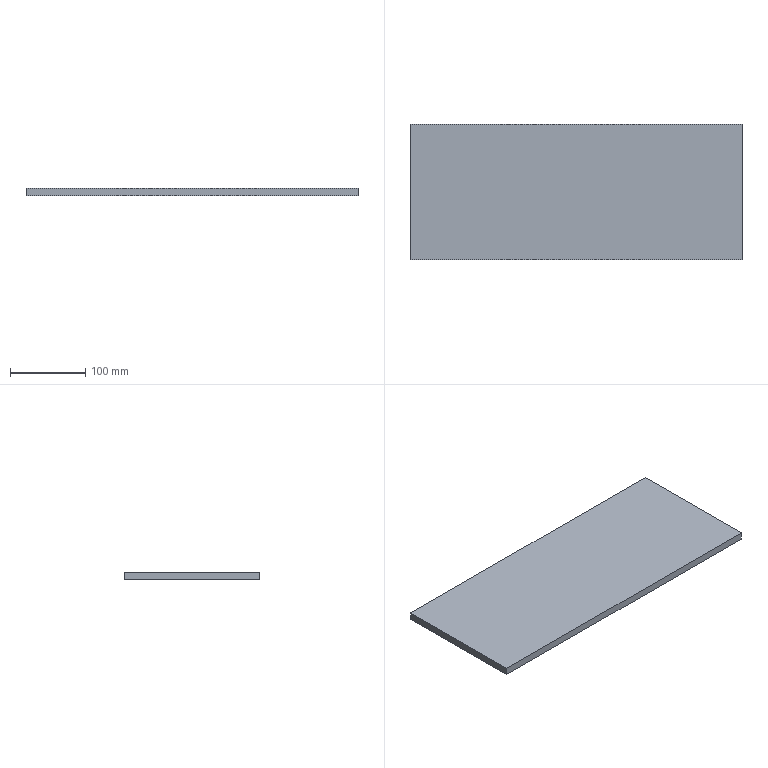Part | SolidWorks | features Extrusion 1 | 1 solid | 6 faces | box 440 x 180 x 10 mm | volume 792000 mm3 | plane 6
STEP:
#1=CARTESIAN_POINT('',(0.,0.,0.));
#2=VERTEX_POINT('',#1);
#3=CARTESIAN_POINT('',(0.,-180.,0.));
#4=VERTEX_POINT('',#3);
#5=CARTESIAN_POINT('',(0.,-180.,0.));
#6=DIRECTION('',(0.,-1.,0.));
#7=VECTOR('',#6,1000.);
#8=LINE('',#5,#7);
#9=EDGE_CURVE('',#2,#4,#8,.T.);
#10=ORIENTED_EDGE('',*,*,#9,.T.);
#11=CARTESIAN_POINT('',(0.,-180.,10.));
#12=VERTEX_POINT('',#11);
#13=CARTESIAN_POINT('',(0.,-180.,10.));
#14=DIRECTION('',(0.,0.,-1.));
#15=VECTOR('',#14,1000.);
#16=LINE('',#13,#15);
#17=EDGE_CURVE('',#12,#4,#16,.T.);
#18=ORIENTED_EDGE('',*,*,#17,.F.);
#19=CARTESIAN_POINT('',(0.,0.,10.));
#20=VERTEX_POINT('',#19);
#21=CARTESIAN_POINT('',(0.,-180.,10.));
#22=DIRECTION('',(0.,-1.,0.));
#23=VECTOR('',#22,1000.);
#24=LINE('',#21,#23);
#25=EDGE_CURVE('',#20,#12,#24,.T.);
#26=ORIENTED_EDGE('',*,*,#25,.F.);
#27=CARTESIAN_POINT('',(0.,0.,10.));
#28=DIRECTION('',(0.,0.,-1.));
#29=VECTOR('',#28,1000.);
#30=LINE('',#27,#29);
#31=EDGE_CURVE('',#20,#2,#30,.T.);
#32=ORIENTED_EDGE('',*,*,#31,.T.);
#33=EDGE_LOOP('',(#10,#18,#26,#32));
#34=FACE_OUTER_BOUND('',#33,.T.);
#35=CARTESIAN_POINT('',(0.,-180.,10.));
#36=DIRECTION('',(1.,0.,0.));
#37=DIRECTION('',(0.,0.,-1.));
#38=AXIS2_PLACEMENT_3D('',#35,#36,#37);
#39=PLANE('',#38);
#40=ADVANCED_FACE('',(#34),#39,.F.);
#41=CARTESIAN_POINT('',(440.,-180.,0.));
#42=VERTEX_POINT('',#41);
#43=CARTESIAN_POINT('',(440.,-180.,0.));
#44=DIRECTION('',(1.,0.,0.));
#45=VECTOR('',#44,1000.);
#46=LINE('',#43,#45);
#47=EDGE_CURVE('',#4,#42,#46,.T.);
#48=ORIENTED_EDGE('',*,*,#47,.T.);
#49=CARTESIAN_POINT('',(440.,-180.,10.));
#50=VERTEX_POINT('',#49);
#51=CARTESIAN_POINT('',(440.,-180.,10.));
#52=DIRECTION('',(0.,0.,-1.));
#53=VECTOR('',#52,1000.);
#54=LINE('',#51,#53);
#55=EDGE_CURVE('',#50,#42,#54,.T.);
#56=ORIENTED_EDGE('',*,*,#55,.F.);
#57=CARTESIAN_POINT('',(440.,-180.,10.));
#58=DIRECTION('',(1.,0.,0.));
#59=VECTOR('',#58,1000.);
#60=LINE('',#57,#59);
#61=EDGE_CURVE('',#12,#50,#60,.T.);
#62=ORIENTED_EDGE('',*,*,#61,.F.);
#63=ORIENTED_EDGE('',*,*,#17,.T.);
#64=EDGE_LOOP('',(#48,#56,#62,#63));
#65=FACE_OUTER_BOUND('',#64,.T.);
#66=CARTESIAN_POINT('',(440.,-180.,10.));
#67=DIRECTION('',(0.,1.,0.));
#68=DIRECTION('',(0.,0.,1.));
#69=AXIS2_PLACEMENT_3D('',#66,#67,#68);
#70=PLANE('',#69);
#71=ADVANCED_FACE('',(#65),#70,.F.);
#72=CARTESIAN_POINT('',(440.,0.,0.));
#73=VERTEX_POINT('',#72);
#74=CARTESIAN_POINT('',(440.,0.,0.));
#75=DIRECTION('',(0.,1.,0.));
#76=VECTOR('',#75,1000.);
#77=LINE('',#74,#76);
#78=EDGE_CURVE('',#42,#73,#77,.T.);
#79=ORIENTED_EDGE('',*,*,#78,.T.);
#80=CARTESIAN_POINT('',(440.,0.,10.));
#81=VERTEX_POINT('',#80);
#82=CARTESIAN_POINT('',(440.,0.,10.));
#83=DIRECTION('',(0.,0.,-1.));
#84=VECTOR('',#83,1000.);
#85=LINE('',#82,#84);
#86=EDGE_CURVE('',#81,#73,#85,.T.);
#87=ORIENTED_EDGE('',*,*,#86,.F.);
#88=CARTESIAN_POINT('',(440.,0.,10.));
#89=DIRECTION('',(0.,1.,0.));
#90=VECTOR('',#89,1000.);
#91=LINE('',#88,#90);
#92=EDGE_CURVE('',#50,#81,#91,.T.);
#93=ORIENTED_EDGE('',*,*,#92,.F.);
#94=ORIENTED_EDGE('',*,*,#55,.T.);
#95=EDGE_LOOP('',(#79,#87,#93,#94));
#96=FACE_OUTER_BOUND('',#95,.T.);
#97=CARTESIAN_POINT('',(440.,0.,10.));
#98=DIRECTION('',(-1.,0.,0.));
#99=DIRECTION('',(0.,0.,1.));
#100=AXIS2_PLACEMENT_3D('',#97,#98,#99);
#101=PLANE('',#100);
#102=ADVANCED_FACE('',(#96),#101,.F.);
#103=CARTESIAN_POINT('',(0.,0.,0.));
#104=DIRECTION('',(-1.,0.,0.));
#105=VECTOR('',#104,1000.);
#106=LINE('',#103,#105);
#107=EDGE_CURVE('',#73,#2,#106,.T.);
#108=ORIENTED_EDGE('',*,*,#107,.T.);
#109=ORIENTED_EDGE('',*,*,#31,.F.);
#110=CARTESIAN_POINT('',(0.,0.,10.));
#111=DIRECTION('',(-1.,0.,0.));
#112=VECTOR('',#111,1000.);
#113=LINE('',#110,#112);
#114=EDGE_CURVE('',#81,#20,#113,.T.);
#115=ORIENTED_EDGE('',*,*,#114,.F.);
#116=ORIENTED_EDGE('',*,*,#86,.T.);
#117=EDGE_LOOP('',(#108,#109,#115,#116));
#118=FACE_OUTER_BOUND('',#117,.T.);
#119=CARTESIAN_POINT('',(0.,0.,10.));
#120=DIRECTION('',(0.,-1.,0.));
#121=DIRECTION('',(0.,0.,-1.));
#122=AXIS2_PLACEMENT_3D('',#119,#120,#121);
#123=PLANE('',#122);
#124=ADVANCED_FACE('',(#118),#123,.F.);
#125=ORIENTED_EDGE('',*,*,#25,.T.);
#126=ORIENTED_EDGE('',*,*,#61,.T.);
#127=ORIENTED_EDGE('',*,*,#92,.T.);
#128=ORIENTED_EDGE('',*,*,#114,.T.);
#129=EDGE_LOOP('',(#125,#126,#127,#128));
#130=FACE_OUTER_BOUND('',#129,.T.);
#131=CARTESIAN_POINT('',(0.,0.,10.));
#132=DIRECTION('',(0.,0.,-1.));
#133=DIRECTION('',(-1.,0.,0.));
#134=AXIS2_PLACEMENT_3D('',#131,#132,#133);
#135=PLANE('',#134);
#136=ADVANCED_FACE('',(#130),#135,.F.);
#137=ORIENTED_EDGE('',*,*,#9,.F.);
#138=ORIENTED_EDGE('',*,*,#107,.F.);
#139=ORIENTED_EDGE('',*,*,#78,.F.);
#140=ORIENTED_EDGE('',*,*,#47,.F.);
#141=EDGE_LOOP('',(#137,#138,#139,#140));
#142=FACE_OUTER_BOUND('',#141,.T.);
#143=CARTESIAN_POINT('',(0.,0.,0.));
#144=DIRECTION('',(0.,0.,-1.));
#145=DIRECTION('',(-1.,0.,0.));
#146=AXIS2_PLACEMENT_3D('',#143,#144,#145);
#147=PLANE('',#146);
#148=ADVANCED_FACE('',(#142),#147,.T.);
#149=CLOSED_SHELL('',(#40,#71,#102,#124,#136,#148));
#150=MANIFOLD_SOLID_BREP('',#149);
#151=CARTESIAN_POINT('',(0.,0.,0.));
#152=DIRECTION('',(0.,0.,1.));
#153=DIRECTION('',(1.,0.,0.));
#154=AXIS2_PLACEMENT_3D('',#151,#152,#153);
#155=(LENGTH_UNIT()NAMED_UNIT(*)SI_UNIT(.MILLI.,.METRE.));
#156=UNCERTAINTY_MEASURE_WITH_UNIT(LENGTH_MEASURE(0.00001),#155,'','');
#157=(NAMED_UNIT(*)PLANE_ANGLE_UNIT()SI_UNIT($,.RADIAN.));
#158=(NAMED_UNIT(*)SI_UNIT($,.STERADIAN.)SOLID_ANGLE_UNIT());
#159=(GEOMETRIC_REPRESENTATION_CONTEXT(3)GLOBAL_UNCERTAINTY_ASSIGNED_CONTEXT((#156))GLOBAL_UNIT_ASSIGNED_CONTEXT((#155,#157,#158))REPRESENTATION_CONTEXT('',''));
#160=ADVANCED_BREP_SHAPE_REPRESENTATION('',(#150,#154),#159);